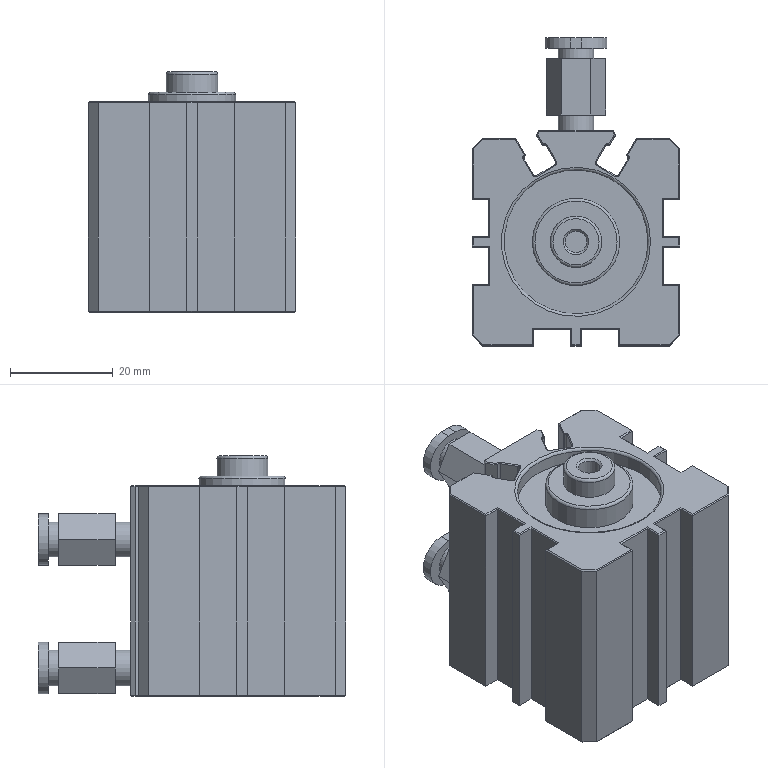Part | STEP file | Tube feed_id942_x_t | 1 solid | 246 faces | box 40.4 x 59.9 x 46.8 mm | volume 59964 mm3 | plane 191 | cylinder 28 | cone 20 | spline 4 | torus 3 | commonest cylinder face diameters 1 x8 10 x5 4.2 x4 7 x4 2 x2 4 x2